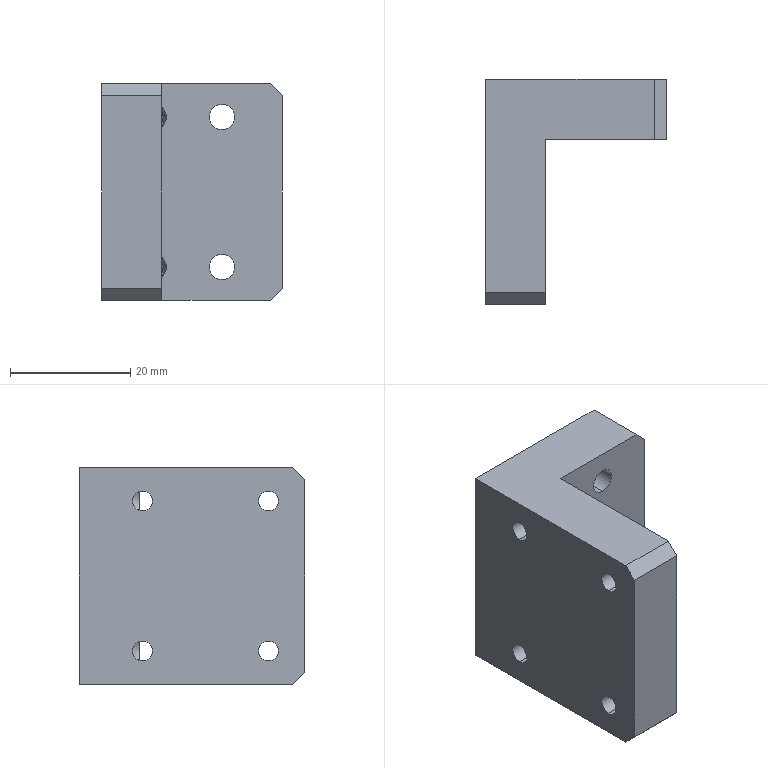Part | SolidWorks | features HoleWzd 2, Chamfer 1, ExtruThin 1 | 1 solid | 26 faces | box 30 x 37.5 x 36 mm | volume 19999 mm3 | cylinder 12 | plane 12 | cone 2 | commonest cylinder face diameters 3.3 x8 4.2 x4
STEP:
#1=CARTESIAN_POINT('',(20.,37.5,-14.6));
#2=VERTEX_POINT('',#1);
#3=CARTESIAN_POINT('',(20.,37.5,-10.4));
#4=VERTEX_POINT('',#3);
#5=CARTESIAN_POINT('',(20.,37.5,-12.5));
#6=DIRECTION('',(0.,1.,0.));
#7=DIRECTION('',(0.,0.,1.));
#8=AXIS2_PLACEMENT_3D('',#5,#6,#7);
#9=CIRCLE('',#8,2.1);
#10=EDGE_CURVE('',#2,#4,#9,.T.);
#11=ORIENTED_EDGE('',*,*,#10,.T.);
#12=CARTESIAN_POINT('',(20.,27.5,-10.4));
#13=VERTEX_POINT('',#12);
#14=CARTESIAN_POINT('',(20.,27.5,-10.4));
#15=DIRECTION('',(0.,-1.,0.));
#16=VECTOR('',#15,1000.);
#17=LINE('',#14,#16);
#18=EDGE_CURVE('',#4,#13,#17,.T.);
#19=ORIENTED_EDGE('',*,*,#18,.T.);
#20=CARTESIAN_POINT('',(20.,27.5,-14.6));
#21=VERTEX_POINT('',#20);
#22=CARTESIAN_POINT('',(20.,27.5,-12.5));
#23=DIRECTION('',(0.,-1.,0.));
#24=DIRECTION('',(0.,0.,-1.));
#25=AXIS2_PLACEMENT_3D('',#22,#23,#24);
#26=CIRCLE('',#25,2.1);
#27=EDGE_CURVE('',#13,#21,#26,.T.);
#28=ORIENTED_EDGE('',*,*,#27,.T.);
#29=CARTESIAN_POINT('',(20.,27.5,-14.6));
#30=DIRECTION('',(0.,-1.,0.));
#31=VECTOR('',#30,1000.);
#32=LINE('',#29,#31);
#33=EDGE_CURVE('',#2,#21,#32,.T.);
#34=ORIENTED_EDGE('',*,*,#33,.F.);
#35=EDGE_LOOP('',(#11,#19,#28,#34));
#36=FACE_OUTER_BOUND('',#35,.T.);
#37=CARTESIAN_POINT('',(20.,27.5,-12.5));
#38=DIRECTION('',(0.,-1.,0.));
#39=DIRECTION('',(0.,0.,-1.));
#40=AXIS2_PLACEMENT_3D('',#37,#38,#39);
#41=CYLINDRICAL_SURFACE('',#40,2.1);
#42=ADVANCED_FACE('',(#36),#41,.F.);
#43=CARTESIAN_POINT('',(20.,37.5,10.4));
#44=VERTEX_POINT('',#43);
#45=CARTESIAN_POINT('',(20.,37.5,14.6));
#46=VERTEX_POINT('',#45);
#47=CARTESIAN_POINT('',(20.,37.5,12.5));
#48=DIRECTION('',(0.,1.,0.));
#49=DIRECTION('',(0.,0.,1.));
#50=AXIS2_PLACEMENT_3D('',#47,#48,#49);
#51=CIRCLE('',#50,2.1);
#52=EDGE_CURVE('',#44,#46,#51,.T.);
#53=ORIENTED_EDGE('',*,*,#52,.T.);
#54=CARTESIAN_POINT('',(20.,27.5,14.6));
#55=VERTEX_POINT('',#54);
#56=CARTESIAN_POINT('',(20.,27.5,14.6));
#57=DIRECTION('',(0.,-1.,0.));
#58=VECTOR('',#57,1000.);
#59=LINE('',#56,#58);
#60=EDGE_CURVE('',#46,#55,#59,.T.);
#61=ORIENTED_EDGE('',*,*,#60,.T.);
#62=CARTESIAN_POINT('',(20.,27.5,10.4));
#63=VERTEX_POINT('',#62);
#64=CARTESIAN_POINT('',(20.,27.5,12.5));
#65=DIRECTION('',(0.,-1.,0.));
#66=DIRECTION('',(0.,0.,-1.));
#67=AXIS2_PLACEMENT_3D('',#64,#65,#66);
#68=CIRCLE('',#67,2.1);
#69=EDGE_CURVE('',#55,#63,#68,.T.);
#70=ORIENTED_EDGE('',*,*,#69,.T.);
#71=CARTESIAN_POINT('',(20.,27.5,10.4));
#72=DIRECTION('',(0.,-1.,0.));
#73=VECTOR('',#72,1000.);
#74=LINE('',#71,#73);
#75=EDGE_CURVE('',#44,#63,#74,.T.);
#76=ORIENTED_EDGE('',*,*,#75,.F.);
#77=EDGE_LOOP('',(#53,#61,#70,#76));
#78=FACE_OUTER_BOUND('',#77,.T.);
#79=CARTESIAN_POINT('',(20.,27.5,12.5));
#80=DIRECTION('',(0.,-1.,0.));
#81=DIRECTION('',(0.,0.,-1.));
#82=AXIS2_PLACEMENT_3D('',#79,#80,#81);
#83=CYLINDRICAL_SURFACE('',#82,2.1);
#84=ADVANCED_FACE('',(#78),#83,.F.);
#85=CARTESIAN_POINT('',(10.,27.,10.85));
#86=VERTEX_POINT('',#85);
#87=CARTESIAN_POINT('',(10.,27.,14.15));
#88=VERTEX_POINT('',#87);
#89=CARTESIAN_POINT('',(10.,27.,12.5));
#90=DIRECTION('',(-1.,0.,0.));
#91=DIRECTION('',(0.,0.,1.));
#92=AXIS2_PLACEMENT_3D('',#89,#90,#91);
#93=CIRCLE('',#92,1.65);
#94=EDGE_CURVE('',#86,#88,#93,.T.);
#95=ORIENTED_EDGE('',*,*,#94,.F.);
#96=CARTESIAN_POINT('',(0.,27.,10.85));
#97=VERTEX_POINT('',#96);
#98=CARTESIAN_POINT('',(0.,27.,10.85));
#99=DIRECTION('',(-1.,0.,0.));
#100=VECTOR('',#99,1000.);
#101=LINE('',#98,#100);
#102=EDGE_CURVE('',#86,#97,#101,.T.);
#103=ORIENTED_EDGE('',*,*,#102,.T.);
#104=CARTESIAN_POINT('',(0.,27.,14.15));
#105=VERTEX_POINT('',#104);
#106=CARTESIAN_POINT('',(0.,27.,12.5));
#107=DIRECTION('',(-1.,0.,0.));
#108=DIRECTION('',(0.,0.,1.));
#109=AXIS2_PLACEMENT_3D('',#106,#107,#108);
#110=CIRCLE('',#109,1.65);
#111=EDGE_CURVE('',#97,#105,#110,.T.);
#112=ORIENTED_EDGE('',*,*,#111,.T.);
#113=CARTESIAN_POINT('',(0.,27.,14.15));
#114=DIRECTION('',(-1.,0.,0.));
#115=VECTOR('',#114,1000.);
#116=LINE('',#113,#115);
#117=EDGE_CURVE('',#88,#105,#116,.T.);
#118=ORIENTED_EDGE('',*,*,#117,.F.);
#119=EDGE_LOOP('',(#95,#103,#112,#118));
#120=FACE_OUTER_BOUND('',#119,.T.);
#121=CARTESIAN_POINT('',(0.,27.,12.5));
#122=DIRECTION('',(-1.,0.,0.));
#123=DIRECTION('',(0.,0.,1.));
#124=AXIS2_PLACEMENT_3D('',#121,#122,#123);
#125=CYLINDRICAL_SURFACE('',#124,1.65);
#126=ADVANCED_FACE('',(#120),#125,.F.);
#127=CARTESIAN_POINT('',(10.,6.,10.85));
#128=VERTEX_POINT('',#127);
#129=CARTESIAN_POINT('',(10.,6.,14.15));
#130=VERTEX_POINT('',#129);
#131=CARTESIAN_POINT('',(10.,6.,12.5));
#132=DIRECTION('',(-1.,0.,0.));
#133=DIRECTION('',(0.,0.,1.));
#134=AXIS2_PLACEMENT_3D('',#131,#132,#133);
#135=CIRCLE('',#134,1.65);
#136=EDGE_CURVE('',#128,#130,#135,.T.);
#137=ORIENTED_EDGE('',*,*,#136,.F.);
#138=CARTESIAN_POINT('',(0.,6.,10.85));
#139=VERTEX_POINT('',#138);
#140=CARTESIAN_POINT('',(0.,6.,10.85));
#141=DIRECTION('',(-1.,0.,0.));
#142=VECTOR('',#141,1000.);
#143=LINE('',#140,#142);
#144=EDGE_CURVE('',#128,#139,#143,.T.);
#145=ORIENTED_EDGE('',*,*,#144,.T.);
#146=CARTESIAN_POINT('',(0.,6.,14.15));
#147=VERTEX_POINT('',#146);
#148=CARTESIAN_POINT('',(0.,6.,12.5));
#149=DIRECTION('',(-1.,0.,0.));
#150=DIRECTION('',(0.,0.,1.));
#151=AXIS2_PLACEMENT_3D('',#148,#149,#150);
#152=CIRCLE('',#151,1.65);
#153=EDGE_CURVE('',#139,#147,#152,.T.);
#154=ORIENTED_EDGE('',*,*,#153,.T.);
#155=CARTESIAN_POINT('',(0.,6.,14.15));
#156=DIRECTION('',(-1.,0.,0.));
#157=VECTOR('',#156,1000.);
#158=LINE('',#155,#157);
#159=EDGE_CURVE('',#130,#147,#158,.T.);
#160=ORIENTED_EDGE('',*,*,#159,.F.);
#161=EDGE_LOOP('',(#137,#145,#154,#160));
#162=FACE_OUTER_BOUND('',#161,.T.);
#163=CARTESIAN_POINT('',(0.,6.,12.5));
#164=DIRECTION('',(-1.,0.,0.));
#165=DIRECTION('',(0.,0.,1.));
#166=AXIS2_PLACEMENT_3D('',#163,#164,#165);
#167=CYLINDRICAL_SURFACE('',#166,1.65);
#168=ADVANCED_FACE('',(#162),#167,.F.);
#169=CARTESIAN_POINT('',(10.,6.,-14.15));
#170=VERTEX_POINT('',#169);
#171=CARTESIAN_POINT('',(10.,6.,-10.85));
#172=VERTEX_POINT('',#171);
#173=CARTESIAN_POINT('',(10.,6.,-12.5));
#174=DIRECTION('',(-1.,0.,0.));
#175=DIRECTION('',(0.,0.,1.));
#176=AXIS2_PLACEMENT_3D('',#173,#174,#175);
#177=CIRCLE('',#176,1.65);
#178=EDGE_CURVE('',#170,#172,#177,.T.);
#179=ORIENTED_EDGE('',*,*,#178,.F.);
#180=CARTESIAN_POINT('',(0.,6.,-14.15));
#181=VERTEX_POINT('',#180);
#182=CARTESIAN_POINT('',(0.,6.,-14.15));
#183=DIRECTION('',(-1.,0.,0.));
#184=VECTOR('',#183,1000.);
#185=LINE('',#182,#184);
#186=EDGE_CURVE('',#170,#181,#185,.T.);
#187=ORIENTED_EDGE('',*,*,#186,.T.);
#188=CARTESIAN_POINT('',(0.,6.,-10.85));
#189=VERTEX_POINT('',#188);
#190=CARTESIAN_POINT('',(0.,6.,-12.5));
#191=DIRECTION('',(-1.,0.,0.));
#192=DIRECTION('',(0.,0.,1.));
#193=AXIS2_PLACEMENT_3D('',#190,#191,#192);
#194=CIRCLE('',#193,1.65);
#195=EDGE_CURVE('',#181,#189,#194,.T.);
#196=ORIENTED_EDGE('',*,*,#195,.T.);
#197=CARTESIAN_POINT('',(0.,6.,-10.85));
#198=DIRECTION('',(-1.,0.,0.));
#199=VECTOR('',#198,1000.);
#200=LINE('',#197,#199);
#201=EDGE_CURVE('',#172,#189,#200,.T.);
#202=ORIENTED_EDGE('',*,*,#201,.F.);
#203=EDGE_LOOP('',(#179,#187,#196,#202));
#204=FACE_OUTER_BOUND('',#203,.T.);
#205=CARTESIAN_POINT('',(0.,6.,-12.5));
#206=DIRECTION('',(-1.,0.,0.));
#207=DIRECTION('',(0.,0.,1.));
#208=AXIS2_PLACEMENT_3D('',#205,#206,#207);
#209=CYLINDRICAL_SURFACE('',#208,1.65);
#210=ADVANCED_FACE('',(#204),#209,.F.);
#211=CARTESIAN_POINT('',(10.,27.,-14.15));
#212=VERTEX_POINT('',#211);
#213=CARTESIAN_POINT('',(10.,27.,-10.85));
#214=VERTEX_POINT('',#213);
#215=CARTESIAN_POINT('',(10.,27.,-12.5));
#216=DIRECTION('',(-1.,0.,0.));
#217=DIRECTION('',(0.,0.,1.));
#218=AXIS2_PLACEMENT_3D('',#215,#216,#217);
#219=CIRCLE('',#218,1.65);
#220=EDGE_CURVE('',#212,#214,#219,.T.);
#221=ORIENTED_EDGE('',*,*,#220,.F.);
#222=CARTESIAN_POINT('',(0.,27.,-14.15));
#223=VERTEX_POINT('',#222);
#224=CARTESIAN_POINT('',(0.,27.,-14.15));
#225=DIRECTION('',(-1.,0.,0.));
#226=VECTOR('',#225,1000.);
#227=LINE('',#224,#226);
#228=EDGE_CURVE('',#212,#223,#227,.T.);
#229=ORIENTED_EDGE('',*,*,#228,.T.);
#230=CARTESIAN_POINT('',(0.,27.,-10.85));
#231=VERTEX_POINT('',#230);
#232=CARTESIAN_POINT('',(0.,27.,-12.5));
#233=DIRECTION('',(-1.,0.,0.));
#234=DIRECTION('',(0.,0.,1.));
#235=AXIS2_PLACEMENT_3D('',#232,#233,#234);
#236=CIRCLE('',#235,1.65);
#237=EDGE_CURVE('',#223,#231,#236,.T.);
#238=ORIENTED_EDGE('',*,*,#237,.T.);
#239=CARTESIAN_POINT('',(0.,27.,-10.85));
#240=DIRECTION('',(-1.,0.,0.));
#241=VECTOR('',#240,1000.);
#242=LINE('',#239,#241);
#243=EDGE_CURVE('',#214,#231,#242,.T.);
#244=ORIENTED_EDGE('',*,*,#243,.F.);
#245=EDGE_LOOP('',(#221,#229,#238,#244));
#246=FACE_OUTER_BOUND('',#245,.T.);
#247=CARTESIAN_POINT('',(0.,27.,-12.5));
#248=DIRECTION('',(-1.,0.,0.));
#249=DIRECTION('',(0.,0.,1.));
#250=AXIS2_PLACEMENT_3D('',#247,#248,#249);
#251=CYLINDRICAL_SURFACE('',#250,1.65);
#252=ADVANCED_FACE('',(#246),#251,.F.);
#253=CARTESIAN_POINT('',(20.,27.5,12.5));
#254=DIRECTION('',(0.,-1.,0.));
#255=DIRECTION('',(0.,0.,-1.));
#256=AXIS2_PLACEMENT_3D('',#253,#254,#255);
#257=CIRCLE('',#256,2.1);
#258=EDGE_CURVE('',#63,#55,#257,.T.);
#259=ORIENTED_EDGE('',*,*,#258,.F.);
#260=ORIENTED_EDGE('',*,*,#69,.F.);
#261=EDGE_LOOP('',(#259,#260));
#262=FACE_BOUND('',#261,.T.);
#263=CARTESIAN_POINT('',(10.1,27.5,14.072));
#264=VERTEX_POINT('',#263);
#265=CARTESIAN_POINT('',(10.1,27.5,10.928));
#266=VERTEX_POINT('',#265);
#267=CARTESIAN_POINT('',(10.1,27.5,14.072));
#268=CARTESIAN_POINT('',(10.243,27.5,13.822));
#269=CARTESIAN_POINT('',(10.385,27.5,13.572));
#270=CARTESIAN_POINT('',(10.582,27.5,13.187));
#271=CARTESIAN_POINT('',(10.646,27.5,13.057));
#272=CARTESIAN_POINT('',(10.724,27.5,12.856));
#273=CARTESIAN_POINT('',(10.747,27.5,12.788));
#274=CARTESIAN_POINT('',(10.781,27.5,12.648));
#275=CARTESIAN_POINT('',(10.791,27.5,12.575));
#276=CARTESIAN_POINT('',(10.791,27.5,12.359));
#277=CARTESIAN_POINT('',(10.752,27.5,12.217));
#278=CARTESIAN_POINT('',(10.648,27.5,11.947));
#279=CARTESIAN_POINT('',(10.584,27.5,11.817));
#280=CARTESIAN_POINT('',(10.387,27.5,11.43));
#281=CARTESIAN_POINT('',(10.244,27.5,11.179));
#282=CARTESIAN_POINT('',(10.1,27.5,10.928));
#283=B_SPLINE_CURVE_WITH_KNOTS('',3,(#267,#268,#269,#270,#271,#272,#273,#274,#275,#276,#277,#278,#279,#280,#281,#282),.UNSPECIFIED.,.F.,.F.,(4,2,2,2,2,2,2,4),(0.007383,0.008248,0.00868,0.008896,0.009112,0.009544,0.009976,0.01084),.UNSPECIFIED.);
#284=EDGE_CURVE('',#264,#266,#283,.T.);
#285=ORIENTED_EDGE('',*,*,#284,.T.);
#286=CARTESIAN_POINT('',(10.,27.5,10.928));
#287=VERTEX_POINT('',#286);
#288=CARTESIAN_POINT('',(0.,27.5,10.928));
#289=DIRECTION('',(-1.,0.,0.));
#290=VECTOR('',#289,1000.);
#291=LINE('',#288,#290);
#292=EDGE_CURVE('',#266,#287,#291,.T.);
#293=ORIENTED_EDGE('',*,*,#292,.T.);
#294=CARTESIAN_POINT('',(10.,27.5,-10.928));
#295=VERTEX_POINT('',#294);
#296=CARTESIAN_POINT('',(10.,27.5,18.));
#297=DIRECTION('',(0.,0.,-1.));
#298=VECTOR('',#297,1000.);
#299=LINE('',#296,#298);
#300=EDGE_CURVE('',#287,#295,#299,.T.);
#301=ORIENTED_EDGE('',*,*,#300,.T.);
#302=CARTESIAN_POINT('',(10.1,27.5,-10.928));
#303=VERTEX_POINT('',#302);
#304=CARTESIAN_POINT('',(0.,27.5,-10.928));
#305=DIRECTION('',(1.,0.,0.));
#306=VECTOR('',#305,1000.);
#307=LINE('',#304,#306);
#308=EDGE_CURVE('',#295,#303,#307,.T.);
#309=ORIENTED_EDGE('',*,*,#308,.T.);
#310=CARTESIAN_POINT('',(10.1,27.5,-14.072));
#311=VERTEX_POINT('',#310);
#312=CARTESIAN_POINT('',(10.1,27.5,-10.928));
#313=CARTESIAN_POINT('',(10.243,27.5,-11.178));
#314=CARTESIAN_POINT('',(10.385,27.5,-11.428));
#315=CARTESIAN_POINT('',(10.582,27.5,-11.813));
#316=CARTESIAN_POINT('',(10.646,27.5,-11.943));
#317=CARTESIAN_POINT('',(10.724,27.5,-12.144));
#318=CARTESIAN_POINT('',(10.747,27.5,-12.212));
#319=CARTESIAN_POINT('',(10.781,27.5,-12.352));
#320=CARTESIAN_POINT('',(10.791,27.5,-12.425));
#321=CARTESIAN_POINT('',(10.791,27.5,-12.641));
#322=CARTESIAN_POINT('',(10.752,27.5,-12.783));
#323=CARTESIAN_POINT('',(10.648,27.5,-13.053));
#324=CARTESIAN_POINT('',(10.584,27.5,-13.183));
#325=CARTESIAN_POINT('',(10.387,27.5,-13.57));
#326=CARTESIAN_POINT('',(10.244,27.5,-13.821));
#327=CARTESIAN_POINT('',(10.1,27.5,-14.072));
#328=B_SPLINE_CURVE_WITH_KNOTS('',3,(#312,#313,#314,#315,#316,#317,#318,#319,#320,#321,#322,#323,#324,#325,#326,#327),.UNSPECIFIED.,.F.,.F.,(4,2,2,2,2,2,2,4),(0.007383,0.008248,0.00868,0.008896,0.009112,0.009544,0.009976,0.01084),.UNSPECIFIED.);
#329=EDGE_CURVE('',#303,#311,#328,.T.);
#330=ORIENTED_EDGE('',*,*,#329,.T.);
#331=CARTESIAN_POINT('',(10.,27.5,-14.072));
#332=VERTEX_POINT('',#331);
#333=CARTESIAN_POINT('',(0.,27.5,-14.072));
#334=DIRECTION('',(-1.,0.,0.));
#335=VECTOR('',#334,1000.);
#336=LINE('',#333,#335);
#337=EDGE_CURVE('',#311,#332,#336,.T.);
#338=ORIENTED_EDGE('',*,*,#337,.T.);
#339=CARTESIAN_POINT('',(10.,27.5,-18.));
#340=VERTEX_POINT('',#339);
#341=CARTESIAN_POINT('',(10.,27.5,18.));
#342=DIRECTION('',(0.,0.,-1.));
#343=VECTOR('',#342,1000.);
#344=LINE('',#341,#343);
#345=EDGE_CURVE('',#332,#340,#344,.T.);
#346=ORIENTED_EDGE('',*,*,#345,.T.);
#347=CARTESIAN_POINT('',(28.,27.5,-18.));
#348=VERTEX_POINT('',#347);
#349=CARTESIAN_POINT('',(0.,27.5,-18.));
#350=DIRECTION('',(1.,0.,0.));
#351=VECTOR('',#350,1000.);
#352=LINE('',#349,#351);
#353=EDGE_CURVE('',#340,#348,#352,.T.);
#354=ORIENTED_EDGE('',*,*,#353,.T.);
#355=CARTESIAN_POINT('',(30.,27.5,-16.));
#356=VERTEX_POINT('',#355);
#357=CARTESIAN_POINT('',(28.,27.5,-18.));
#358=DIRECTION('',(0.7071,0.,0.7071));
#359=VECTOR('',#358,1000.);
#360=LINE('',#357,#359);
#361=EDGE_CURVE('',#348,#356,#360,.T.);
#362=ORIENTED_EDGE('',*,*,#361,.T.);
#363=CARTESIAN_POINT('',(30.,27.5,16.));
#364=VERTEX_POINT('',#363);
#365=CARTESIAN_POINT('',(30.,27.5,18.));
#366=DIRECTION('',(0.,0.,-1.));
#367=VECTOR('',#366,1000.);
#368=LINE('',#365,#367);
#369=EDGE_CURVE('',#364,#356,#368,.T.);
#370=ORIENTED_EDGE('',*,*,#369,.F.);
#371=CARTESIAN_POINT('',(28.,27.5,18.));
#372=VERTEX_POINT('',#371);
#373=CARTESIAN_POINT('',(30.,27.5,16.));
#374=DIRECTION('',(-0.7071,0.,0.7071));
#375=VECTOR('',#374,1000.);
#376=LINE('',#373,#375);
#377=EDGE_CURVE('',#364,#372,#376,.T.);
#378=ORIENTED_EDGE('',*,*,#377,.T.);
#379=CARTESIAN_POINT('',(10.,27.5,18.));
#380=VERTEX_POINT('',#379);
#381=CARTESIAN_POINT('',(0.,27.5,18.));
#382=DIRECTION('',(1.,0.,0.));
#383=VECTOR('',#382,1000.);
#384=LINE('',#381,#383);
#385=EDGE_CURVE('',#380,#372,#384,.T.);
#386=ORIENTED_EDGE('',*,*,#385,.F.);
#387=CARTESIAN_POINT('',(10.,27.5,14.072));
#388=VERTEX_POINT('',#387);
#389=CARTESIAN_POINT('',(10.,27.5,18.));
#390=DIRECTION('',(0.,0.,-1.));
#391=VECTOR('',#390,1000.);
#392=LINE('',#389,#391);
#393=EDGE_CURVE('',#380,#388,#392,.T.);
#394=ORIENTED_EDGE('',*,*,#393,.T.);
#395=CARTESIAN_POINT('',(0.,27.5,14.072));
#396=DIRECTION('',(1.,0.,0.));
#397=VECTOR('',#396,1000.);
#398=LINE('',#395,#397);
#399=EDGE_CURVE('',#388,#264,#398,.T.);
#400=ORIENTED_EDGE('',*,*,#399,.T.);
#401=EDGE_LOOP('',(#285,#293,#301,#309,#330,#338,#346,#354,#362,#370,#378,#386,#394,#400));
#402=FACE_OUTER_BOUND('',#401,.T.);
#403=CARTESIAN_POINT('',(20.,27.5,-12.5));
#404=DIRECTION('',(0.,-1.,0.));
#405=DIRECTION('',(0.,0.,-1.));
#406=AXIS2_PLACEMENT_3D('',#403,#404,#405);
#407=CIRCLE('',#406,2.1);
#408=EDGE_CURVE('',#21,#13,#407,.T.);
#409=ORIENTED_EDGE('',*,*,#408,.F.);
#410=ORIENTED_EDGE('',*,*,#27,.F.);
#411=EDGE_LOOP('',(#409,#410));
#412=FACE_BOUND('',#411,.T.);
#413=CARTESIAN_POINT('',(0.,27.5,18.));
#414=DIRECTION('',(0.,1.,0.));
#415=DIRECTION('',(0.,0.,1.));
#416=AXIS2_PLACEMENT_3D('',#413,#414,#415);
#417=PLANE('',#416);
#418=ADVANCED_FACE('',(#262,#402,#412),#417,.F.);
#419=CARTESIAN_POINT('',(30.,37.5,16.));
#420=VERTEX_POINT('',#419);
#421=CARTESIAN_POINT('',(30.,37.5,-16.));
#422=VERTEX_POINT('',#421);
#423=CARTESIAN_POINT('',(30.,37.5,18.));
#424=DIRECTION('',(0.,0.,-1.));
#425=VECTOR('',#424,1000.);
#426=LINE('',#423,#425);
#427=EDGE_CURVE('',#420,#422,#426,.T.);
#428=ORIENTED_EDGE('',*,*,#427,.F.);
#429=CARTESIAN_POINT('',(30.,27.5,16.));
#430=DIRECTION('',(0.,-1.,0.));
#431=VECTOR('',#430,1000.);
#432=LINE('',#429,#431);
#433=EDGE_CURVE('',#420,#364,#432,.T.);
#434=ORIENTED_EDGE('',*,*,#433,.T.);
#435=ORIENTED_EDGE('',*,*,#369,.T.);
#436=CARTESIAN_POINT('',(30.,37.5,-16.));
#437=DIRECTION('',(0.,1.,0.));
#438=VECTOR('',#437,1000.);
#439=LINE('',#436,#438);
#440=EDGE_CURVE('',#356,#422,#439,.T.);
#441=ORIENTED_EDGE('',*,*,#440,.T.);
#442=EDGE_LOOP('',(#428,#434,#435,#441));
#443=FACE_OUTER_BOUND('',#442,.T.);
#444=CARTESIAN_POINT('',(30.,37.5,18.));
#445=DIRECTION('',(1.,0.,0.));
#446=DIRECTION('',(0.,0.,-1.));
#447=AXIS2_PLACEMENT_3D('',#444,#445,#446);
#448=PLANE('',#447);
#449=ADVANCED_FACE('',(#443),#448,.T.);
#450=ORIENTED_EDGE('',*,*,#10,.F.);
#451=CARTESIAN_POINT('',(20.,37.5,-12.5));
#452=DIRECTION('',(0.,1.,0.));
#453=DIRECTION('',(0.,0.,1.));
#454=AXIS2_PLACEMENT_3D('',#451,#452,#453);
#455=CIRCLE('',#454,2.1);
#456=EDGE_CURVE('',#4,#2,#455,.T.);
#457=ORIENTED_EDGE('',*,*,#456,.F.);
#458=EDGE_LOOP('',(#450,#457));
#459=FACE_BOUND('',#458,.T.);
#460=ORIENTED_EDGE('',*,*,#52,.F.);
#461=CARTESIAN_POINT('',(20.,37.5,12.5));
#462=DIRECTION('',(0.,1.,0.));
#463=DIRECTION('',(0.,0.,1.));
#464=AXIS2_PLACEMENT_3D('',#461,#462,#463);
#465=CIRCLE('',#464,2.1);
#466=EDGE_CURVE('',#46,#44,#465,.T.);
#467=ORIENTED_EDGE('',*,*,#466,.F.);
#468=EDGE_LOOP('',(#460,#467));
#469=FACE_BOUND('',#468,.T.);
#470=CARTESIAN_POINT('',(0.,37.5,18.));
#471=VERTEX_POINT('',#470);
#472=CARTESIAN_POINT('',(28.,37.5,18.));
#473=VERTEX_POINT('',#472);
#474=CARTESIAN_POINT('',(0.,37.5,18.));
#475=DIRECTION('',(1.,0.,0.));
#476=VECTOR('',#475,1000.);
#477=LINE('',#474,#476);
#478=EDGE_CURVE('',#471,#473,#477,.T.);
#479=ORIENTED_EDGE('',*,*,#478,.T.);
#480=CARTESIAN_POINT('',(14.,37.5,32.));
#481=DIRECTION('',(0.7071,0.,-0.7071));
#482=VECTOR('',#481,1000.);
#483=LINE('',#480,#482);
#484=EDGE_CURVE('',#473,#420,#483,.T.);
#485=ORIENTED_EDGE('',*,*,#484,.T.);
#486=ORIENTED_EDGE('',*,*,#427,.T.);
#487=CARTESIAN_POINT('',(28.,37.5,-18.));
#488=VERTEX_POINT('',#487);
#489=CARTESIAN_POINT('',(32.,37.5,-14.));
#490=DIRECTION('',(-0.7071,0.,-0.7071));
#491=VECTOR('',#490,1000.);
#492=LINE('',#489,#491);
#493=EDGE_CURVE('',#422,#488,#492,.T.);
#494=ORIENTED_EDGE('',*,*,#493,.T.);
#495=CARTESIAN_POINT('',(0.,37.5,-18.));
#496=VERTEX_POINT('',#495);
#497=CARTESIAN_POINT('',(0.,37.5,-18.));
#498=DIRECTION('',(1.,0.,0.));
#499=VECTOR('',#498,1000.);
#500=LINE('',#497,#499);
#501=EDGE_CURVE('',#496,#488,#500,.T.);
#502=ORIENTED_EDGE('',*,*,#501,.F.);
#503=CARTESIAN_POINT('',(0.,37.5,18.));
#504=DIRECTION('',(0.,0.,-1.));
#505=VECTOR('',#504,1000.);
#506=LINE('',#503,#505);
#507=EDGE_CURVE('',#471,#496,#506,.T.);
#508=ORIENTED_EDGE('',*,*,#507,.F.);
#509=EDGE_LOOP('',(#479,#485,#486,#494,#502,#508));
#510=FACE_OUTER_BOUND('',#509,.T.);
#511=CARTESIAN_POINT('',(0.,37.5,18.));
#512=DIRECTION('',(0.,1.,0.));
#513=DIRECTION('',(0.,0.,1.));
#514=AXIS2_PLACEMENT_3D('',#511,#512,#513);
#515=PLANE('',#514);
#516=ADVANCED_FACE('',(#459,#469,#510),#515,.T.);
#517=CARTESIAN_POINT('',(0.,27.,12.5));
#518=DIRECTION('',(-1.,0.,0.));
#519=DIRECTION('',(0.,0.,1.));
#520=AXIS2_PLACEMENT_3D('',#517,#518,#519);
#521=CIRCLE('',#520,1.65);
#522=EDGE_CURVE('',#105,#97,#521,.T.);
#523=ORIENTED_EDGE('',*,*,#522,.F.);
#524=ORIENTED_EDGE('',*,*,#111,.F.);
#525=EDGE_LOOP('',(#523,#524));
#526=FACE_BOUND('',#525,.T.);
#527=CARTESIAN_POINT('',(0.,6.,12.5));
#528=DIRECTION('',(-1.,0.,0.));
#529=DIRECTION('',(0.,0.,1.));
#530=AXIS2_PLACEMENT_3D('',#527,#528,#529);
#531=CIRCLE('',#530,1.65);
#532=EDGE_CURVE('',#147,#139,#531,.T.);
#533=ORIENTED_EDGE('',*,*,#532,.F.);
#534=ORIENTED_EDGE('',*,*,#153,.F.);
#535=EDGE_LOOP('',(#533,#534));
#536=FACE_BOUND('',#535,.T.);
#537=CARTESIAN_POINT('',(0.,6.,-12.5));
#538=DIRECTION('',(-1.,0.,0.));
#539=DIRECTION('',(0.,0.,1.));
#540=AXIS2_PLACEMENT_3D('',#537,#538,#539);
#541=CIRCLE('',#540,1.65);
#542=EDGE_CURVE('',#189,#181,#541,.T.);
#543=ORIENTED_EDGE('',*,*,#542,.F.);
#544=ORIENTED_EDGE('',*,*,#195,.F.);
#545=EDGE_LOOP('',(#543,#544));
#546=FACE_BOUND('',#545,.T.);
#547=CARTESIAN_POINT('',(0.,27.,-12.5));
#548=DIRECTION('',(-1.,0.,0.));
#549=DIRECTION('',(0.,0.,1.));
#550=AXIS2_PLACEMENT_3D('',#547,#548,#549);
#551=CIRCLE('',#550,1.65);
#552=EDGE_CURVE('',#231,#223,#551,.T.);
#553=ORIENTED_EDGE('',*,*,#552,.F.);
#554=ORIENTED_EDGE('',*,*,#237,.F.);
#555=EDGE_LOOP('',(#553,#554));
#556=FACE_BOUND('',#555,.T.);
#557=CARTESIAN_POINT('',(0.,0.,16.));
#558=VERTEX_POINT('',#557);
#559=CARTESIAN_POINT('',(0.,0.,-16.));
#560=VERTEX_POINT('',#559);
#561=CARTESIAN_POINT('',(0.,0.,18.));
#562=DIRECTION('',(0.,0.,-1.));
#563=VECTOR('',#562,1000.);
#564=LINE('',#561,#563);
#565=EDGE_CURVE('',#558,#560,#564,.T.);
#566=ORIENTED_EDGE('',*,*,#565,.F.);
#567=CARTESIAN_POINT('',(0.,2.,18.));
#568=VERTEX_POINT('',#567);
#569=CARTESIAN_POINT('',(0.,1.,17.));
#570=DIRECTION('',(0.,0.7071,0.7071));
#571=VECTOR('',#570,1000.);
#572=LINE('',#569,#571);
#573=EDGE_CURVE('',#558,#568,#572,.T.);
#574=ORIENTED_EDGE('',*,*,#573,.T.);
#575=CARTESIAN_POINT('',(0.,0.,18.));
#576=DIRECTION('',(0.,1.,0.));
#577=VECTOR('',#576,1000.);
#578=LINE('',#575,#577);
#579=EDGE_CURVE('',#568,#471,#578,.T.);
#580=ORIENTED_EDGE('',*,*,#579,.T.);
#581=ORIENTED_EDGE('',*,*,#507,.T.);
#582=CARTESIAN_POINT('',(0.,2.,-18.));
#583=VERTEX_POINT('',#582);
#584=CARTESIAN_POINT('',(0.,0.,-18.));
#585=DIRECTION('',(0.,1.,0.));
#586=VECTOR('',#585,1000.);
#587=LINE('',#584,#586);
#588=EDGE_CURVE('',#583,#496,#587,.T.);
#589=ORIENTED_EDGE('',*,*,#588,.F.);
#590=CARTESIAN_POINT('',(0.,-17.,1.));
#591=DIRECTION('',(0.,-0.7071,0.7071));
#592=VECTOR('',#591,1000.);
#593=LINE('',#590,#592);
#594=EDGE_CURVE('',#583,#560,#593,.T.);
#595=ORIENTED_EDGE('',*,*,#594,.T.);
#596=EDGE_LOOP('',(#566,#574,#580,#581,#589,#595));
#597=FACE_OUTER_BOUND('',#596,.T.);
#598=CARTESIAN_POINT('',(0.,0.,18.));
#599=DIRECTION('',(-1.,0.,0.));
#600=DIRECTION('',(0.,0.,1.));
#601=AXIS2_PLACEMENT_3D('',#598,#599,#600);
#602=PLANE('',#601);
#603=ADVANCED_FACE('',(#526,#536,#546,#556,#597),#602,.T.);
#604=CARTESIAN_POINT('',(10.,0.,16.));
#605=VERTEX_POINT('',#604);
#606=CARTESIAN_POINT('',(10.,0.,-16.));
#607=VERTEX_POINT('',#606);
#608=CARTESIAN_POINT('',(10.,0.,18.));
#609=DIRECTION('',(0.,0.,-1.));
#610=VECTOR('',#609,1000.);
#611=LINE('',#608,#610);
#612=EDGE_CURVE('',#605,#607,#611,.T.);
#613=ORIENTED_EDGE('',*,*,#612,.F.);
#614=CARTESIAN_POINT('',(0.,0.,16.));
#615=DIRECTION('',(-1.,0.,0.));
#616=VECTOR('',#615,1000.);
#617=LINE('',#614,#616);
#618=EDGE_CURVE('',#605,#558,#617,.T.);
#619=ORIENTED_EDGE('',*,*,#618,.T.);
#620=ORIENTED_EDGE('',*,*,#565,.T.);
#621=CARTESIAN_POINT('',(10.,0.,-16.));
#622=DIRECTION('',(1.,0.,0.));
#623=VECTOR('',#622,1000.);
#624=LINE('',#621,#623);
#625=EDGE_CURVE('',#560,#607,#624,.T.);
#626=ORIENTED_EDGE('',*,*,#625,.T.);
#627=EDGE_LOOP('',(#613,#619,#620,#626));
#628=FACE_OUTER_BOUND('',#627,.T.);
#629=CARTESIAN_POINT('',(10.,0.,18.));
#630=DIRECTION('',(0.,-1.,0.));
#631=DIRECTION('',(0.,0.,-1.));
#632=AXIS2_PLACEMENT_3D('',#629,#630,#631);
#633=PLANE('',#632);
#634=ADVANCED_FACE('',(#628),#633,.T.);
#635=CARTESIAN_POINT('',(10.,6.,12.5));
#636=DIRECTION('',(-1.,0.,0.));
#637=DIRECTION('',(0.,0.,1.));
#638=AXIS2_PLACEMENT_3D('',#635,#636,#637);
#639=CIRCLE('',#638,1.65);
#640=EDGE_CURVE('',#130,#128,#639,.T.);
#641=ORIENTED_EDGE('',*,*,#640,.T.);
#642=ORIENTED_EDGE('',*,*,#136,.T.);
#643=EDGE_LOOP('',(#641,#642));
#644=FACE_BOUND('',#643,.T.);
#645=CARTESIAN_POINT('',(10.,6.,-12.5));
#646=DIRECTION('',(-1.,0.,0.));
#647=DIRECTION('',(0.,0.,1.));
#648=AXIS2_PLACEMENT_3D('',#645,#646,#647);
#649=CIRCLE('',#648,1.65);
#650=EDGE_CURVE('',#172,#170,#649,.T.);
#651=ORIENTED_EDGE('',*,*,#650,.T.);
#652=ORIENTED_EDGE('',*,*,#178,.T.);
#653=EDGE_LOOP('',(#651,#652));
#654=FACE_BOUND('',#653,.T.);
#655=ORIENTED_EDGE('',*,*,#300,.F.);
#656=CARTESIAN_POINT('',(10.,27.,12.5));
#657=DIRECTION('',(-1.,0.,0.));
#658=DIRECTION('',(0.,0.,1.));
#659=AXIS2_PLACEMENT_3D('',#656,#657,#658);
#660=CIRCLE('',#659,1.65);
#661=EDGE_CURVE('',#287,#86,#660,.T.);
#662=ORIENTED_EDGE('',*,*,#661,.T.);
#663=ORIENTED_EDGE('',*,*,#94,.T.);
#664=CARTESIAN_POINT('',(10.,27.,12.5));
#665=DIRECTION('',(-1.,0.,0.));
#666=DIRECTION('',(0.,0.,1.));
#667=AXIS2_PLACEMENT_3D('',#664,#665,#666);
#668=CIRCLE('',#667,1.65);
#669=EDGE_CURVE('',#88,#388,#668,.T.);
#670=ORIENTED_EDGE('',*,*,#669,.T.);
#671=ORIENTED_EDGE('',*,*,#393,.F.);
#672=CARTESIAN_POINT('',(10.,2.,18.));
#673=VERTEX_POINT('',#672);
#674=CARTESIAN_POINT('',(10.,0.,18.));
#675=DIRECTION('',(0.,1.,0.));
#676=VECTOR('',#675,1000.);
#677=LINE('',#674,#676);
#678=EDGE_CURVE('',#673,#380,#677,.T.);
#679=ORIENTED_EDGE('',*,*,#678,.F.);
#680=CARTESIAN_POINT('',(10.,0.,16.));
#681=DIRECTION('',(0.,-0.7071,-0.7071));
#682=VECTOR('',#681,1000.);
#683=LINE('',#680,#682);
#684=EDGE_CURVE('',#673,#605,#683,.T.);
#685=ORIENTED_EDGE('',*,*,#684,.T.);
#686=ORIENTED_EDGE('',*,*,#612,.T.);
#687=CARTESIAN_POINT('',(10.,2.,-18.));
#688=VERTEX_POINT('',#687);
#689=CARTESIAN_POINT('',(10.,2.,-18.));
#690=DIRECTION('',(0.,0.7071,-0.7071));
#691=VECTOR('',#690,1000.);
#692=LINE('',#689,#691);
#693=EDGE_CURVE('',#607,#688,#692,.T.);
#694=ORIENTED_EDGE('',*,*,#693,.T.);
#695=CARTESIAN_POINT('',(10.,0.,-18.));
#696=DIRECTION('',(0.,1.,0.));
#697=VECTOR('',#696,1000.);
#698=LINE('',#695,#697);
#699=EDGE_CURVE('',#688,#340,#698,.T.);
#700=ORIENTED_EDGE('',*,*,#699,.T.);
#701=ORIENTED_EDGE('',*,*,#345,.F.);
#702=CARTESIAN_POINT('',(10.,27.,-12.5));
#703=DIRECTION('',(-1.,0.,0.));
#704=DIRECTION('',(0.,0.,1.));
#705=AXIS2_PLACEMENT_3D('',#702,#703,#704);
#706=CIRCLE('',#705,1.65);
#707=EDGE_CURVE('',#332,#212,#706,.T.);
#708=ORIENTED_EDGE('',*,*,#707,.T.);
#709=ORIENTED_EDGE('',*,*,#220,.T.);
#710=CARTESIAN_POINT('',(10.,27.,-12.5));
#711=DIRECTION('',(-1.,0.,0.));
#712=DIRECTION('',(0.,0.,1.));
#713=AXIS2_PLACEMENT_3D('',#710,#711,#712);
#714=CIRCLE('',#713,1.65);
#715=EDGE_CURVE('',#214,#295,#714,.T.);
#716=ORIENTED_EDGE('',*,*,#715,.T.);
#717=EDGE_LOOP('',(#655,#662,#663,#670,#671,#679,#685,#686,#694,#700,#701,#708,#709,#716));
#718=FACE_OUTER_BOUND('',#717,.T.);
#719=CARTESIAN_POINT('',(10.,0.,18.));
#720=DIRECTION('',(-1.,0.,0.));
#721=DIRECTION('',(0.,0.,1.));
#722=AXIS2_PLACEMENT_3D('',#719,#720,#721);
#723=PLANE('',#722);
#724=ADVANCED_FACE('',(#644,#654,#718),#723,.F.);
#725=ORIENTED_EDGE('',*,*,#579,.F.);
#726=CARTESIAN_POINT('',(10.,2.,18.));
#727=DIRECTION('',(1.,0.,0.));
#728=VECTOR('',#727,1000.);
#729=LINE('',#726,#728);
#730=EDGE_CURVE('',#568,#673,#729,.T.);
#731=ORIENTED_EDGE('',*,*,#730,.T.);
#732=ORIENTED_EDGE('',*,*,#678,.T.);
#733=ORIENTED_EDGE('',*,*,#385,.T.);
#734=CARTESIAN_POINT('',(28.,37.5,18.));
#735=DIRECTION('',(0.,1.,0.));
#736=VECTOR('',#735,1000.);
#737=LINE('',#734,#736);
#738=EDGE_CURVE('',#372,#473,#737,.T.);
#739=ORIENTED_EDGE('',*,*,#738,.T.);
#740=ORIENTED_EDGE('',*,*,#478,.F.);
#741=EDGE_LOOP('',(#725,#731,#732,#733,#739,#740));
#742=FACE_OUTER_BOUND('',#741,.T.);
#743=CARTESIAN_POINT('',(0.,0.,18.));
#744=DIRECTION('',(0.,0.,-1.));
#745=DIRECTION('',(-1.,0.,0.));
#746=AXIS2_PLACEMENT_3D('',#743,#744,#745);
#747=PLANE('',#746);
#748=ADVANCED_FACE('',(#742),#747,.F.);
#749=ORIENTED_EDGE('',*,*,#501,.T.);
#750=CARTESIAN_POINT('',(28.,0.,-18.));
#751=DIRECTION('',(0.,-1.,0.));
#752=VECTOR('',#751,1000.);
#753=LINE('',#750,#752);
#754=EDGE_CURVE('',#488,#348,#753,.T.);
#755=ORIENTED_EDGE('',*,*,#754,.T.);
#756=ORIENTED_EDGE('',*,*,#353,.F.);
#757=ORIENTED_EDGE('',*,*,#699,.F.);
#758=CARTESIAN_POINT('',(0.,2.,-18.));
#759=DIRECTION('',(-1.,0.,0.));
#760=VECTOR('',#759,1000.);
#761=LINE('',#758,#760);
#762=EDGE_CURVE('',#688,#583,#761,.T.);
#763=ORIENTED_EDGE('',*,*,#762,.T.);
#764=ORIENTED_EDGE('',*,*,#588,.T.);
#765=EDGE_LOOP('',(#749,#755,#756,#757,#763,#764));
#766=FACE_OUTER_BOUND('',#765,.T.);
#767=CARTESIAN_POINT('',(0.,0.,-18.));
#768=DIRECTION('',(0.,0.,-1.));
#769=DIRECTION('',(-1.,0.,0.));
#770=AXIS2_PLACEMENT_3D('',#767,#768,#769);
#771=PLANE('',#770);
#772=ADVANCED_FACE('',(#766),#771,.T.);
#773=ORIENTED_EDGE('',*,*,#684,.F.);
#774=ORIENTED_EDGE('',*,*,#730,.F.);
#775=ORIENTED_EDGE('',*,*,#573,.F.);
#776=ORIENTED_EDGE('',*,*,#618,.F.);
#777=EDGE_LOOP('',(#773,#774,#775,#776));
#778=FACE_OUTER_BOUND('',#777,.T.);
#779=CARTESIAN_POINT('',(10.,0.,16.));
#780=DIRECTION('',(0.,-0.7071,0.7071));
#781=DIRECTION('',(1.,0.,0.));
#782=AXIS2_PLACEMENT_3D('',#779,#780,#781);
#783=PLANE('',#782);
#784=ADVANCED_FACE('',(#778),#783,.T.);
#785=ORIENTED_EDGE('',*,*,#484,.F.);
#786=ORIENTED_EDGE('',*,*,#738,.F.);
#787=ORIENTED_EDGE('',*,*,#377,.F.);
#788=ORIENTED_EDGE('',*,*,#433,.F.);
#789=EDGE_LOOP('',(#785,#786,#787,#788));
#790=FACE_OUTER_BOUND('',#789,.T.);
#791=CARTESIAN_POINT('',(30.,37.5,16.));
#792=DIRECTION('',(0.7071,0.,0.7071));
#793=DIRECTION('',(0.,1.,0.));
#794=AXIS2_PLACEMENT_3D('',#791,#792,#793);
#795=PLANE('',#794);
#796=ADVANCED_FACE('',(#790),#795,.T.);
#797=ORIENTED_EDGE('',*,*,#493,.F.);
#798=ORIENTED_EDGE('',*,*,#440,.F.);
#799=ORIENTED_EDGE('',*,*,#361,.F.);
#800=ORIENTED_EDGE('',*,*,#754,.F.);
#801=EDGE_LOOP('',(#797,#798,#799,#800));
#802=FACE_OUTER_BOUND('',#801,.T.);
#803=CARTESIAN_POINT('',(28.,0.,-18.));
#804=DIRECTION('',(-0.7071,0.,0.7071));
#805=DIRECTION('',(0.,-1.,0.));
#806=AXIS2_PLACEMENT_3D('',#803,#804,#805);
#807=PLANE('',#806);
#808=ADVANCED_FACE('',(#802),#807,.F.);
#809=ORIENTED_EDGE('',*,*,#693,.F.);
#810=ORIENTED_EDGE('',*,*,#625,.F.);
#811=ORIENTED_EDGE('',*,*,#594,.F.);
#812=ORIENTED_EDGE('',*,*,#762,.F.);
#813=EDGE_LOOP('',(#809,#810,#811,#812));
#814=FACE_OUTER_BOUND('',#813,.T.);
#815=CARTESIAN_POINT('',(0.,2.,-18.));
#816=DIRECTION('',(0.,0.7071,0.7071));
#817=DIRECTION('',(-1.,0.,0.));
#818=AXIS2_PLACEMENT_3D('',#815,#816,#817);
#819=PLANE('',#818);
#820=ADVANCED_FACE('',(#814),#819,.F.);
#821=ORIENTED_EDGE('',*,*,#228,.F.);
#822=ORIENTED_EDGE('',*,*,#707,.F.);
#823=ORIENTED_EDGE('',*,*,#337,.F.);
#824=CARTESIAN_POINT('',(10.1,27.,-12.5));
#825=DIRECTION('',(-1.,0.,0.));
#826=DIRECTION('',(0.,0.,1.));
#827=AXIS2_PLACEMENT_3D('',#824,#825,#826);
#828=CIRCLE('',#827,1.65);
#829=EDGE_CURVE('',#303,#311,#828,.T.);
#830=ORIENTED_EDGE('',*,*,#829,.F.);
#831=ORIENTED_EDGE('',*,*,#308,.F.);
#832=ORIENTED_EDGE('',*,*,#715,.F.);
#833=ORIENTED_EDGE('',*,*,#243,.T.);
#834=ORIENTED_EDGE('',*,*,#552,.T.);
#835=EDGE_LOOP('',(#821,#822,#823,#830,#831,#832,#833,#834));
#836=FACE_OUTER_BOUND('',#835,.T.);
#837=CARTESIAN_POINT('',(0.,27.,-12.5));
#838=DIRECTION('',(-1.,0.,0.));
#839=DIRECTION('',(0.,0.,1.));
#840=AXIS2_PLACEMENT_3D('',#837,#838,#839);
#841=CYLINDRICAL_SURFACE('',#840,1.65);
#842=ADVANCED_FACE('',(#836),#841,.F.);
#843=ORIENTED_EDGE('',*,*,#829,.T.);
#844=ORIENTED_EDGE('',*,*,#329,.F.);
#845=EDGE_LOOP('',(#843,#844));
#846=FACE_OUTER_BOUND('',#845,.T.);
#847=CARTESIAN_POINT('',(10.1,27.,-12.5));
#848=DIRECTION('',(-1.,0.,0.));
#849=DIRECTION('',(0.,0.,1.));
#850=AXIS2_PLACEMENT_3D('',#847,#848,#849);
#851=CONICAL_SURFACE('',#850,1.65,1.03);
#852=ADVANCED_FACE('',(#846),#851,.F.);
#853=ORIENTED_EDGE('',*,*,#186,.F.);
#854=ORIENTED_EDGE('',*,*,#650,.F.);
#855=ORIENTED_EDGE('',*,*,#201,.T.);
#856=ORIENTED_EDGE('',*,*,#542,.T.);
#857=EDGE_LOOP('',(#853,#854,#855,#856));
#858=FACE_OUTER_BOUND('',#857,.T.);
#859=CARTESIAN_POINT('',(0.,6.,-12.5));
#860=DIRECTION('',(-1.,0.,0.));
#861=DIRECTION('',(0.,0.,1.));
#862=AXIS2_PLACEMENT_3D('',#859,#860,#861);
#863=CYLINDRICAL_SURFACE('',#862,1.65);
#864=ADVANCED_FACE('',(#858),#863,.F.);
#865=ORIENTED_EDGE('',*,*,#144,.F.);
#866=ORIENTED_EDGE('',*,*,#640,.F.);
#867=ORIENTED_EDGE('',*,*,#159,.T.);
#868=ORIENTED_EDGE('',*,*,#532,.T.);
#869=EDGE_LOOP('',(#865,#866,#867,#868));
#870=FACE_OUTER_BOUND('',#869,.T.);
#871=CARTESIAN_POINT('',(0.,6.,12.5));
#872=DIRECTION('',(-1.,0.,0.));
#873=DIRECTION('',(0.,0.,1.));
#874=AXIS2_PLACEMENT_3D('',#871,#872,#873);
#875=CYLINDRICAL_SURFACE('',#874,1.65);
#876=ADVANCED_FACE('',(#870),#875,.F.);
#877=ORIENTED_EDGE('',*,*,#102,.F.);
#878=ORIENTED_EDGE('',*,*,#661,.F.);
#879=ORIENTED_EDGE('',*,*,#292,.F.);
#880=CARTESIAN_POINT('',(10.1,27.,12.5));
#881=DIRECTION('',(-1.,0.,0.));
#882=DIRECTION('',(0.,0.,1.));
#883=AXIS2_PLACEMENT_3D('',#880,#881,#882);
#884=CIRCLE('',#883,1.65);
#885=EDGE_CURVE('',#264,#266,#884,.T.);
#886=ORIENTED_EDGE('',*,*,#885,.F.);
#887=ORIENTED_EDGE('',*,*,#399,.F.);
#888=ORIENTED_EDGE('',*,*,#669,.F.);
#889=ORIENTED_EDGE('',*,*,#117,.T.);
#890=ORIENTED_EDGE('',*,*,#522,.T.);
#891=EDGE_LOOP('',(#877,#878,#879,#886,#887,#888,#889,#890));
#892=FACE_OUTER_BOUND('',#891,.T.);
#893=CARTESIAN_POINT('',(0.,27.,12.5));
#894=DIRECTION('',(-1.,0.,0.));
#895=DIRECTION('',(0.,0.,1.));
#896=AXIS2_PLACEMENT_3D('',#893,#894,#895);
#897=CYLINDRICAL_SURFACE('',#896,1.65);
#898=ADVANCED_FACE('',(#892),#897,.F.);
#899=ORIENTED_EDGE('',*,*,#885,.T.);
#900=ORIENTED_EDGE('',*,*,#284,.F.);
#901=EDGE_LOOP('',(#899,#900));
#902=FACE_OUTER_BOUND('',#901,.T.);
#903=CARTESIAN_POINT('',(10.1,27.,12.5));
#904=DIRECTION('',(-1.,0.,0.));
#905=DIRECTION('',(0.,0.,1.));
#906=AXIS2_PLACEMENT_3D('',#903,#904,#905);
#907=CONICAL_SURFACE('',#906,1.65,1.03);
#908=ADVANCED_FACE('',(#902),#907,.F.);
#909=ORIENTED_EDGE('',*,*,#60,.F.);
#910=ORIENTED_EDGE('',*,*,#466,.T.);
#911=ORIENTED_EDGE('',*,*,#75,.T.);
#912=ORIENTED_EDGE('',*,*,#258,.T.);
#913=EDGE_LOOP('',(#909,#910,#911,#912));
#914=FACE_OUTER_BOUND('',#913,.T.);
#915=CARTESIAN_POINT('',(20.,27.5,12.5));
#916=DIRECTION('',(0.,-1.,0.));
#917=DIRECTION('',(0.,0.,-1.));
#918=AXIS2_PLACEMENT_3D('',#915,#916,#917);
#919=CYLINDRICAL_SURFACE('',#918,2.1);
#920=ADVANCED_FACE('',(#914),#919,.F.);
#921=ORIENTED_EDGE('',*,*,#18,.F.);
#922=ORIENTED_EDGE('',*,*,#456,.T.);
#923=ORIENTED_EDGE('',*,*,#33,.T.);
#924=ORIENTED_EDGE('',*,*,#408,.T.);
#925=EDGE_LOOP('',(#921,#922,#923,#924));
#926=FACE_OUTER_BOUND('',#925,.T.);
#927=CARTESIAN_POINT('',(20.,27.5,-12.5));
#928=DIRECTION('',(0.,-1.,0.));
#929=DIRECTION('',(0.,0.,-1.));
#930=AXIS2_PLACEMENT_3D('',#927,#928,#929);
#931=CYLINDRICAL_SURFACE('',#930,2.1);
#932=ADVANCED_FACE('',(#926),#931,.F.);
#933=CLOSED_SHELL('',(#42,#84,#126,#168,#210,#252,#418,#449,#516,#603,#634,#724,#748,#772,#784,#796,#808,#820,#842,#852,#864,#876,#898,#908,#920,#932));
#934=MANIFOLD_SOLID_BREP('',#933);
#935=CARTESIAN_POINT('',(0.,0.,0.));
#936=DIRECTION('',(0.,0.,1.));
#937=DIRECTION('',(1.,0.,0.));
#938=AXIS2_PLACEMENT_3D('',#935,#936,#937);
#939=(LENGTH_UNIT()NAMED_UNIT(*)SI_UNIT(.MILLI.,.METRE.));
#940=UNCERTAINTY_MEASURE_WITH_UNIT(LENGTH_MEASURE(0.00001),#939,'','');
#941=(NAMED_UNIT(*)PLANE_ANGLE_UNIT()SI_UNIT($,.RADIAN.));
#942=(NAMED_UNIT(*)SI_UNIT($,.STERADIAN.)SOLID_ANGLE_UNIT());
#943=(GEOMETRIC_REPRESENTATION_CONTEXT(3)GLOBAL_UNCERTAINTY_ASSIGNED_CONTEXT((#940))GLOBAL_UNIT_ASSIGNED_CONTEXT((#939,#941,#942))REPRESENTATION_CONTEXT('',''));
#944=ADVANCED_BREP_SHAPE_REPRESENTATION('',(#934,#938),#943);